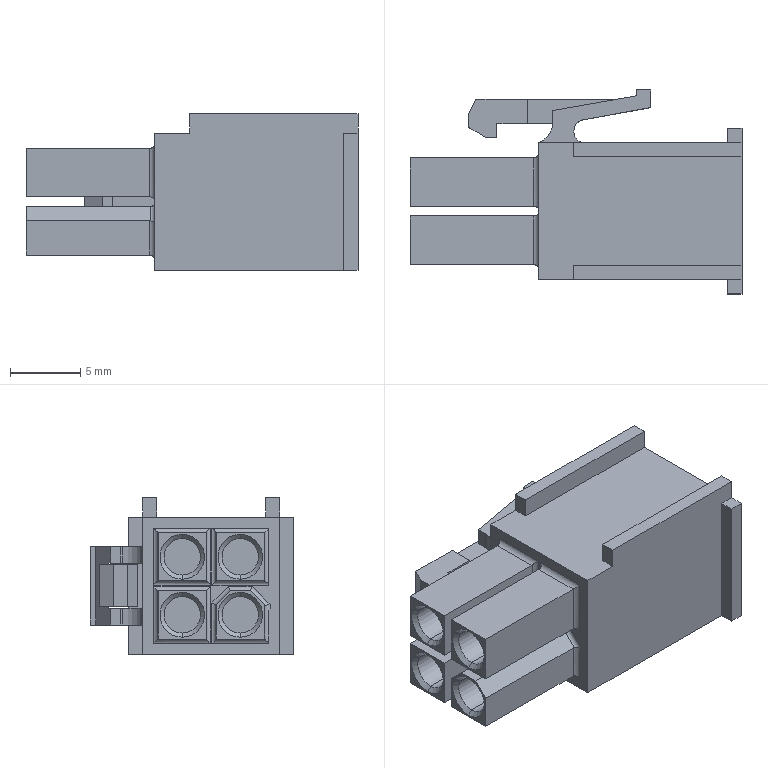Part | STEP file | Motor_Connector_2 | 1 solid | 197 faces | box 23.7 x 14.55 x 11.2 mm | volume 1255 mm3 | plane 138 | cylinder 43 | cone 16 | commonest cylinder face diameters 0.6 x10 0.8 x8 1.82 x8 2.6 x8 1.5 x5 3.1 x4